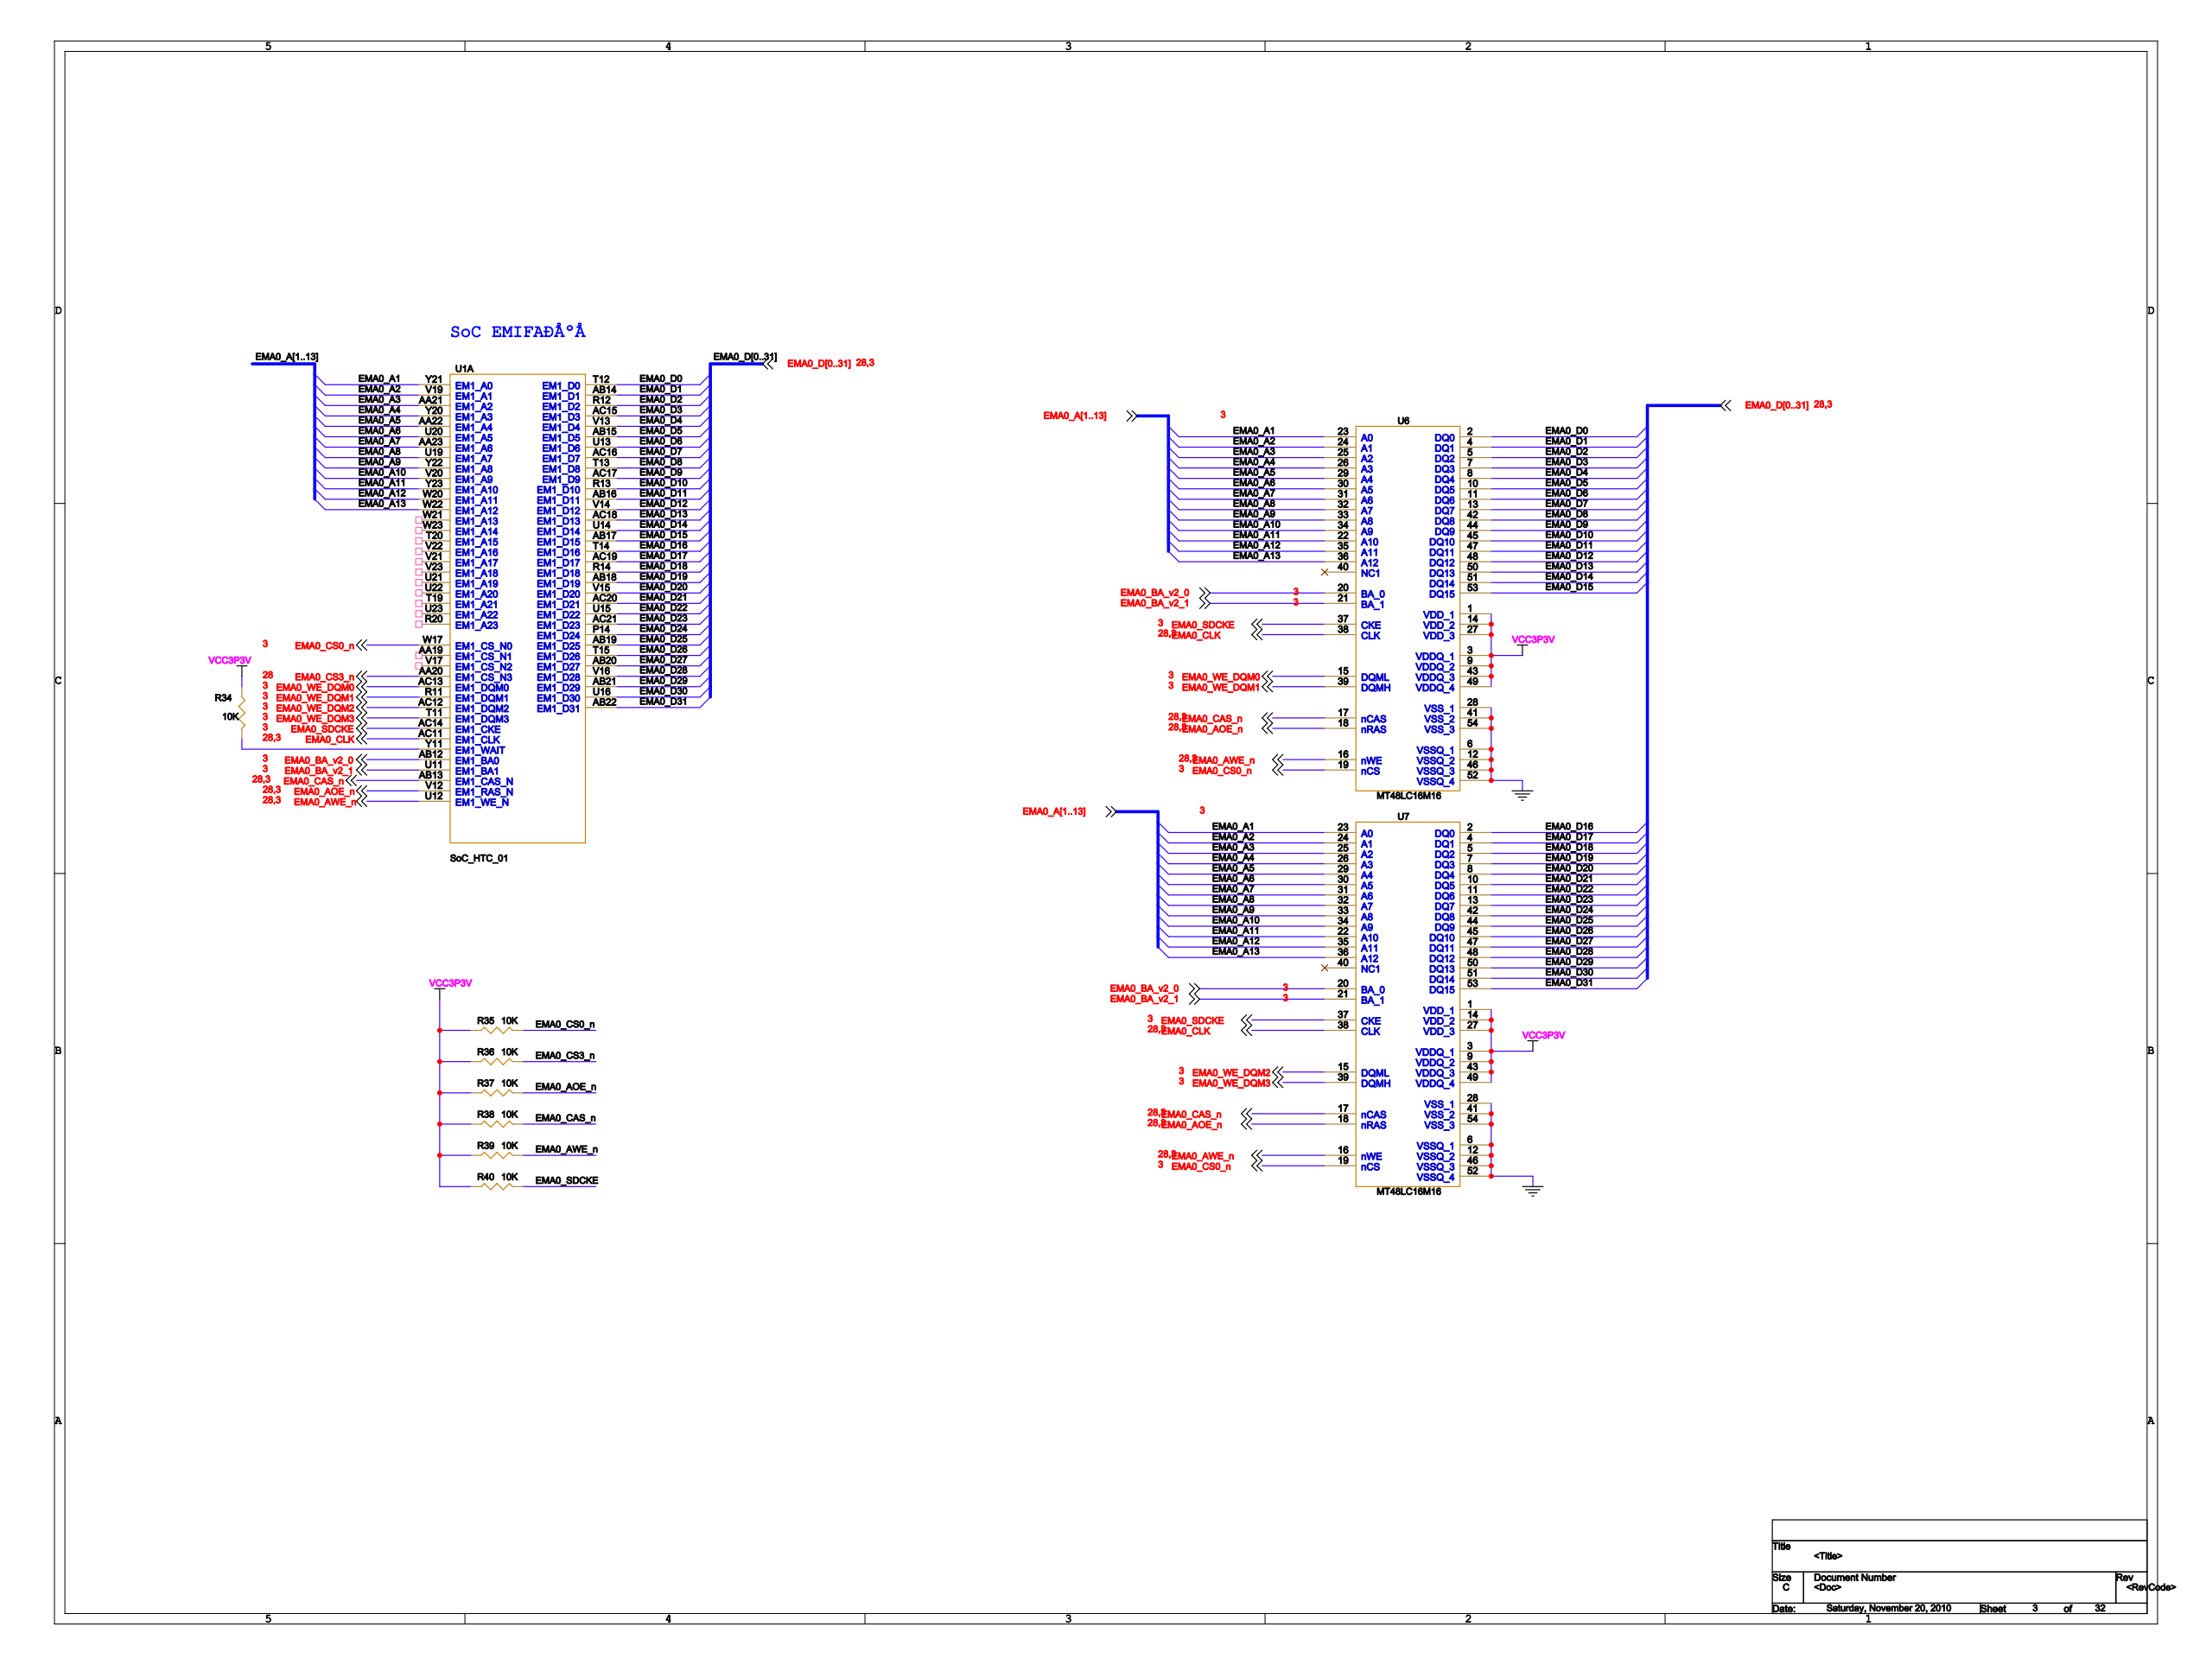Circuit board | Cadence Allegro | 1001 parts | 1318 nets | one sheet of the schematic
Parts on this sheet (reference | value | footprint):
R34 | 10K | 0603
R35 | 10K | 0603
R36 | 10K | 0603
R37 | 10K | 0603
R38 | 10K | 0603
R39 | 10K | 0603
R40 | 10K | 0603
U1 | SoC_HTC_01 | L529_XIN
U6 | MT48LC16M16 | TSOP54
U7 | MT48LC16M16 | TSOP54
U11 | MT48LC32M16 | TSOP54
U14 | MT48LC16M16 | TSOP54
U15 | MT48LC16M16 | TSOP54
U20 | MT48LC16M16 | TSOP54
U21 | MT48LC16M16 | TSOP54
U23 | MT48LC32M16 | TSOP54
Nets of these parts (net: part-pin ...):
EMA0_AOE_N: R37-2 U1-V12 U6-18 U7-18
EMA0_AWE_N: R39-2 U1-U12 U6-16 U7-16
EMA0_D6: U1-U13 U6-11
EMA0_D10: U1-R13 U6-45
EMA0_D8: U1-T13 U6-42
EMA0_D3: U1-AC15 U6-7
EMA0_D18: U1-R14 U7-5
EMA0_D5: U1-AB15 U6-10
EMA0_D26: U1-T15 U7-45
EMA0_D1: U1-AB14 U6-4
EMA0_D20: U1-V15 U7-8
EMA0_D22: U1-U15 U7-11
EMA0_D30: U1-U16 U7-51
EMA0_D28: U1-V16 U7-48
EMA0_CS3_N: R36-2 U1-AA20
EMA0_D7: U1-AC16 U6-13
EMA0_D2: U1-R12 U6-5
EMA0_D24: U1-P14 U7-42
EMA0_D4: U1-V13 U6-8
EMA0_D14: U1-U14 U6-51
EMA0_D0: U1-T12 U6-2
EMA0_D16: U1-T14 U7-2
EMA0_D27: U1-AB20 U7-47
EMA0_CAS_N: R38-2 U1-AB13 U6-17 U7-17
EMA0_D23: U1-AC21 U7-13
EMA0_D11: U1-AB16 U6-47
EMA0_D12: U1-V14 U6-48
EMA0_D25: U1-AB19 U7-44
EMA0_D17: U1-AC19 U7-4
EMA0_D19: U1-AB18 U7-7
EMA0_D15: U1-AB17 U6-53
EMA0_D31: U1-AB22 U7-53
EMA0_D21: U1-AC20 U7-10
EMA0_D13: U1-AC18 U6-50
EMA0_D9: U1-AC17 U6-44
EMA0_D29: U1-AB21 U7-50
EMA0_CLK: U1-AC11 U6-38 U7-38
VCC3P3V: R34-2 R35-1 R36-1 R37-1 R38-1 R39-1 R40-1 U6-1 U6-3 U6-9 U6-14 U6-27 U6-43 U6-49 U7-1 U7-3 U7-9 U7-14 U7-27 U7-43 U7-49 U11-1 U11-3 U11-9 U11-14 U11-27 U11-43 U11-49 U14-1 U14-3 U14-9 U14-14 U14-27 U14-43 U14-49 U15-1 U15-3 U15-9 U15-14 U15-27 U15-43 U15-49 U20-1 U20-3 U20-9 U20-14 U20-27 U20-43 U20-49 U21-1 U21-3 U21-9 U21-14 U21-27 U21-43 U21-49 U23-1 U23-3 U23-9 U23-14 U23-27 U23-43 U23-49
EMA0_A1: U1-Y21 U6-23 U7-23
EMA0_A2: U1-V19 U6-24 U7-24
EMA0_A11: U1-Y23 U6-22 U7-22
EMA0_A12: U1-W20 U6-35 U7-35
EMA0_A13: U1-W22 U6-36 U7-36
EMA0_A3: U1-AA21 U6-25 U7-25
EMA0_A4: U1-Y20 U6-26 U7-26
EMA0_A5: U1-AA22 U6-29 U7-29
EMA0_A6: U1-U20 U6-30 U7-30
EMA0_A7: U1-AA23 U6-31 U7-31
EMA0_A8: U1-U19 U6-32 U7-32
EMA0_A9: U1-Y22 U6-33 U7-33
EMA0_A10: U1-V20 U6-34 U7-34
EMA0_SDCKE: R40-2 U1-AC14 U6-37 U7-37
EMA0_CS0_N: R35-2 U1-W17 U6-19 U7-19
EMA0_WE_DQM0: U1-AC13 U6-15
EMA0_WE_DQM1: U1-R11 U6-39
EMA0_WE_DQM2: U1-AC12 U7-15
EMA0_WE_DQM3: U1-T11 U7-39
N16270293: R34-1 U1-Y11